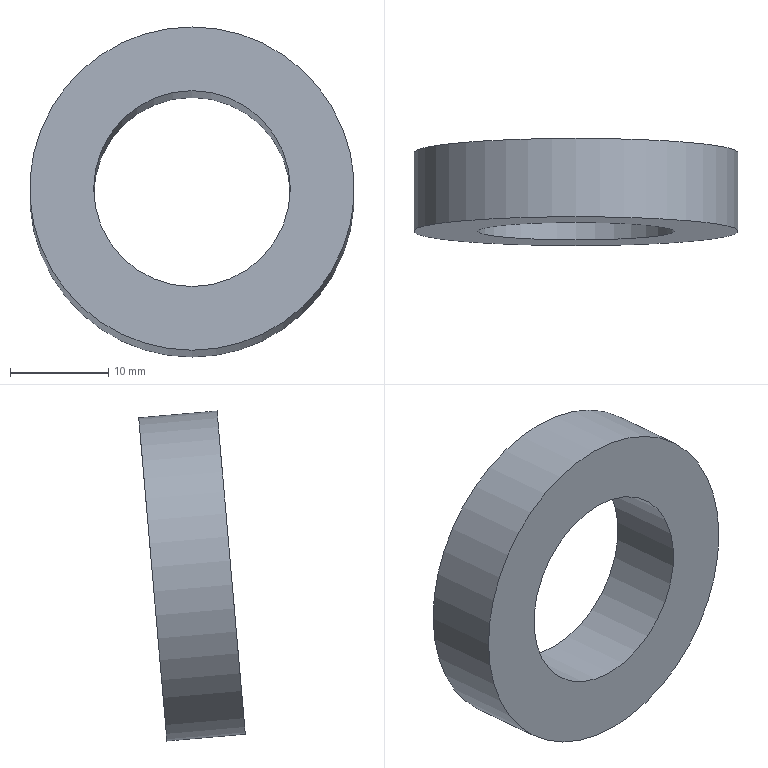Part | NX | features solid 2 | 1 solid | 4 faces | box 33 x 10.846 x 33.572 mm | volume 4329 mm3 | cylinder 2 | plane 2 | commonest cylinder face diameters 20 x1 33 x1
STEP:
#1=CARTESIAN_POINT('',(-322.976,-70.779,-19.654));
#2=VERTEX_POINT('',#1);
#3=CARTESIAN_POINT('',(-322.976,-72.217,-36.092));
#4=DIRECTION('',(0.,0.9962,-0.08716));
#5=DIRECTION('',(0.,0.08716,0.9962));
#6=AXIS2_PLACEMENT_3D('',#3,#4,#5);
#7=CIRCLE('',#6,16.5);
#8=EDGE_CURVE('',#2,#2,#7,.F.);
#9=ORIENTED_EDGE('',*,*,#8,.T.);
#10=EDGE_LOOP('',(#9));
#11=FACE_BOUND('',#10,.T.);
#12=CARTESIAN_POINT('',(-322.976,-78.748,-18.957));
#13=VERTEX_POINT('',#12);
#14=CARTESIAN_POINT('',(-322.976,-80.186,-35.394));
#15=DIRECTION('',(0.,0.9962,-0.08716));
#16=DIRECTION('',(0.,0.08716,0.9962));
#17=AXIS2_PLACEMENT_3D('',#14,#15,#16);
#18=CIRCLE('',#17,16.5);
#19=EDGE_CURVE('',#13,#13,#18,.F.);
#20=ORIENTED_EDGE('',*,*,#19,.F.);
#21=EDGE_LOOP('',(#20));
#22=FACE_BOUND('',#21,.T.);
#23=CARTESIAN_POINT('',(-322.976,-72.217,-36.092));
#24=DIRECTION('',(0.,-0.9962,0.08716));
#25=DIRECTION('',(0.,-0.08716,-0.9962));
#26=AXIS2_PLACEMENT_3D('',#23,#24,#25);
#27=CYLINDRICAL_SURFACE('',#26,16.5);
#28=ADVANCED_FACE('',(#11,#22),#27,.T.);
#29=CARTESIAN_POINT('',(-322.976,-71.345,-26.13));
#30=VERTEX_POINT('',#29);
#31=CARTESIAN_POINT('',(-322.976,-72.217,-36.092));
#32=DIRECTION('',(0.,0.9962,-0.08716));
#33=DIRECTION('',(0.,0.08716,0.9962));
#34=AXIS2_PLACEMENT_3D('',#31,#32,#33);
#35=CIRCLE('',#34,10.);
#36=EDGE_CURVE('',#30,#30,#35,.F.);
#37=ORIENTED_EDGE('',*,*,#36,.F.);
#38=EDGE_LOOP('',(#37));
#39=FACE_BOUND('',#38,.T.);
#40=CARTESIAN_POINT('',(-322.976,-79.315,-25.432));
#41=VERTEX_POINT('',#40);
#42=CARTESIAN_POINT('',(-322.976,-80.186,-35.394));
#43=DIRECTION('',(0.,0.9962,-0.08716));
#44=DIRECTION('',(0.,0.08716,0.9962));
#45=AXIS2_PLACEMENT_3D('',#42,#43,#44);
#46=CIRCLE('',#45,10.);
#47=EDGE_CURVE('',#41,#41,#46,.F.);
#48=ORIENTED_EDGE('',*,*,#47,.T.);
#49=EDGE_LOOP('',(#48));
#50=FACE_BOUND('',#49,.T.);
#51=CARTESIAN_POINT('',(-322.976,-72.217,-36.092));
#52=DIRECTION('',(0.,-0.9962,0.08716));
#53=DIRECTION('',(0.,-0.08716,-0.9962));
#54=AXIS2_PLACEMENT_3D('',#51,#52,#53);
#55=CYLINDRICAL_SURFACE('',#54,10.);
#56=ADVANCED_FACE('',(#39,#50),#55,.F.);
#57=ORIENTED_EDGE('',*,*,#8,.F.);
#58=EDGE_LOOP('',(#57));
#59=FACE_BOUND('',#58,.T.);
#60=ORIENTED_EDGE('',*,*,#36,.T.);
#61=EDGE_LOOP('',(#60));
#62=FACE_BOUND('',#61,.T.);
#63=CARTESIAN_POINT('',(-322.976,-72.217,-36.092));
#64=DIRECTION('',(0.,0.9962,-0.08716));
#65=DIRECTION('',(-1.,0.,0.));
#66=AXIS2_PLACEMENT_3D('',#63,#64,#65);
#67=PLANE('',#66);
#68=ADVANCED_FACE('',(#59,#62),#67,.T.);
#69=ORIENTED_EDGE('',*,*,#19,.T.);
#70=EDGE_LOOP('',(#69));
#71=FACE_BOUND('',#70,.T.);
#72=ORIENTED_EDGE('',*,*,#47,.F.);
#73=EDGE_LOOP('',(#72));
#74=FACE_BOUND('',#73,.T.);
#75=CARTESIAN_POINT('',(-322.976,-80.186,-35.394));
#76=DIRECTION('',(0.,0.9962,-0.08716));
#77=DIRECTION('',(-1.,0.,0.));
#78=AXIS2_PLACEMENT_3D('',#75,#76,#77);
#79=PLANE('',#78);
#80=ADVANCED_FACE('',(#71,#74),#79,.F.);
#81=CLOSED_SHELL('',(#28,#56,#68,#80));
#82=MANIFOLD_SOLID_BREP('',#81);
#83=(LENGTH_UNIT()NAMED_UNIT(*)SI_UNIT(.MILLI.,.METRE.));
#84=UNCERTAINTY_MEASURE_WITH_UNIT(LENGTH_MEASURE(0.00001),#83,'','');
#85=(NAMED_UNIT(*)PLANE_ANGLE_UNIT()SI_UNIT($,.RADIAN.));
#86=(NAMED_UNIT(*)SI_UNIT($,.STERADIAN.)SOLID_ANGLE_UNIT());
#87=(GEOMETRIC_REPRESENTATION_CONTEXT(3)GLOBAL_UNCERTAINTY_ASSIGNED_CONTEXT((#84))GLOBAL_UNIT_ASSIGNED_CONTEXT((#83,#85,#86))REPRESENTATION_CONTEXT('',''));
#88=ADVANCED_BREP_SHAPE_REPRESENTATION('',(#82),#87);